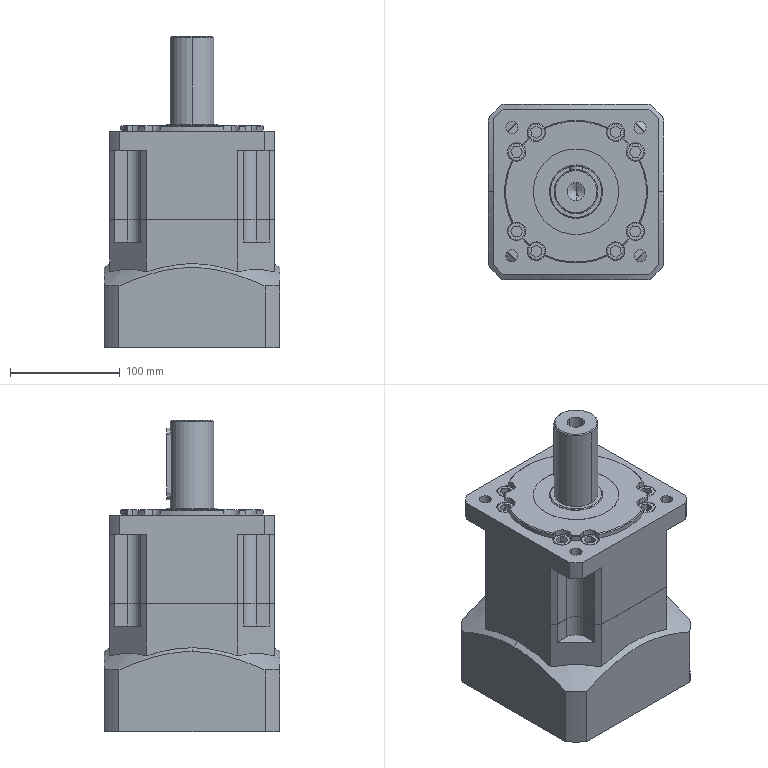Part | SolidWorks | features ICE 18, CirPattern 4, Fillet 2, Revolution 2, Chamfer 1, RevCut 1 | 2 solids | 330 faces | box 160 x 160 x 283 mm | volume 4310215 mm3 | plane 179 | cylinder 110 | torus 24 | cone 17 | commonest cylinder face diameters 16.5 x16 16.8 x16 12 x11 130 x9 8 x8 11 x8